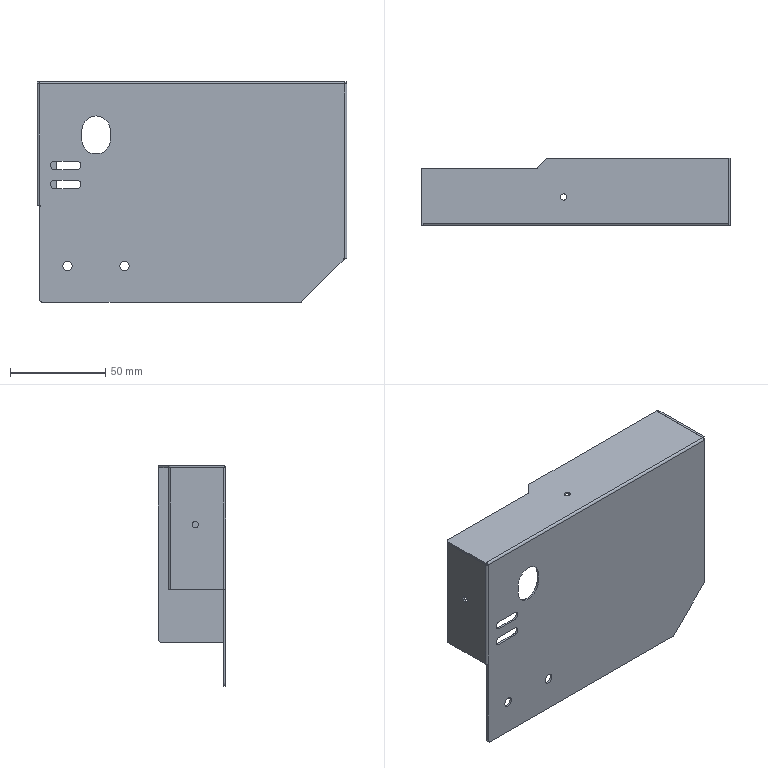Part | STEP file | sprocket guard | 1 solid | 84 faces | box 163 x 35.5 x 116 mm | volume 28902 mm3 | plane 54 | cylinder 30 | commonest cylinder face diameters 0.1 x4 2 x4 2.1 x4 3.3 x4 4.5 x4 5 x4